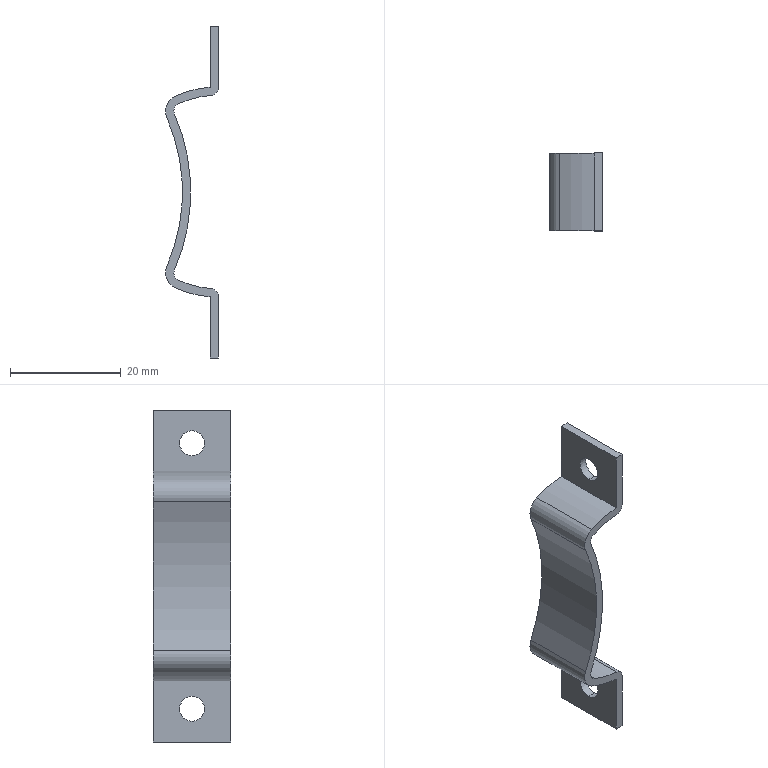Part | SolidWorks | features ExtruThin 1, ICE 1 | 1 solid | 24 faces | box 9.547 x 14 x 60 mm | volume 1466 mm3 | cylinder 16 | plane 8 | commonest cylinder face diameters 3 x4 4.5 x4 6 x2 35 x2 38 x2 67 x1
STEP:
#1=CARTESIAN_POINT('',(-1.5,7.,-26.25));
#2=VERTEX_POINT('',#1);
#3=CARTESIAN_POINT('',(-1.5,7.,-21.75));
#4=VERTEX_POINT('',#3);
#5=CARTESIAN_POINT('',(-1.5,7.,-24.));
#6=DIRECTION('',(-1.,0.,0.));
#7=DIRECTION('',(0.,0.,-1.));
#8=AXIS2_PLACEMENT_3D('',#5,#6,#7);
#9=CIRCLE('',#8,2.25);
#10=EDGE_CURVE('',#2,#4,#9,.T.);
#11=ORIENTED_EDGE('',*,*,#10,.T.);
#12=CARTESIAN_POINT('',(0.,7.,-21.75));
#13=VERTEX_POINT('',#12);
#14=CARTESIAN_POINT('',(-9.548,7.,-21.75));
#15=DIRECTION('',(1.,0.,0.));
#16=VECTOR('',#15,1000.);
#17=LINE('',#14,#16);
#18=EDGE_CURVE('',#4,#13,#17,.T.);
#19=ORIENTED_EDGE('',*,*,#18,.T.);
#20=CARTESIAN_POINT('',(0.,7.,-26.25));
#21=VERTEX_POINT('',#20);
#22=CARTESIAN_POINT('',(0.,7.,-24.));
#23=DIRECTION('',(1.,0.,0.));
#24=DIRECTION('',(0.,0.,-1.));
#25=AXIS2_PLACEMENT_3D('',#22,#23,#24);
#26=CIRCLE('',#25,2.25);
#27=EDGE_CURVE('',#13,#21,#26,.T.);
#28=ORIENTED_EDGE('',*,*,#27,.T.);
#29=CARTESIAN_POINT('',(-9.548,7.,-26.25));
#30=DIRECTION('',(1.,0.,0.));
#31=VECTOR('',#30,1000.);
#32=LINE('',#29,#31);
#33=EDGE_CURVE('',#2,#21,#32,.T.);
#34=ORIENTED_EDGE('',*,*,#33,.F.);
#35=EDGE_LOOP('',(#11,#19,#28,#34));
#36=FACE_OUTER_BOUND('',#35,.T.);
#37=CARTESIAN_POINT('',(-9.548,7.,-24.));
#38=DIRECTION('',(1.,0.,0.));
#39=DIRECTION('',(0.,0.,-1.));
#40=AXIS2_PLACEMENT_3D('',#37,#38,#39);
#41=CYLINDRICAL_SURFACE('',#40,2.25);
#42=ADVANCED_FACE('',(#36),#41,.F.);
#43=CARTESIAN_POINT('',(-1.5,7.,21.75));
#44=VERTEX_POINT('',#43);
#45=CARTESIAN_POINT('',(-1.5,7.,26.25));
#46=VERTEX_POINT('',#45);
#47=CARTESIAN_POINT('',(-1.5,7.,24.));
#48=DIRECTION('',(-1.,0.,0.));
#49=DIRECTION('',(0.,0.,-1.));
#50=AXIS2_PLACEMENT_3D('',#47,#48,#49);
#51=CIRCLE('',#50,2.25);
#52=EDGE_CURVE('',#44,#46,#51,.T.);
#53=ORIENTED_EDGE('',*,*,#52,.T.);
#54=CARTESIAN_POINT('',(0.,7.,26.25));
#55=VERTEX_POINT('',#54);
#56=CARTESIAN_POINT('',(-9.548,7.,26.25));
#57=DIRECTION('',(1.,0.,0.));
#58=VECTOR('',#57,1000.);
#59=LINE('',#56,#58);
#60=EDGE_CURVE('',#46,#55,#59,.T.);
#61=ORIENTED_EDGE('',*,*,#60,.T.);
#62=CARTESIAN_POINT('',(0.,7.,21.75));
#63=VERTEX_POINT('',#62);
#64=CARTESIAN_POINT('',(0.,7.,24.));
#65=DIRECTION('',(1.,0.,0.));
#66=DIRECTION('',(0.,0.,-1.));
#67=AXIS2_PLACEMENT_3D('',#64,#65,#66);
#68=CIRCLE('',#67,2.25);
#69=EDGE_CURVE('',#55,#63,#68,.T.);
#70=ORIENTED_EDGE('',*,*,#69,.T.);
#71=CARTESIAN_POINT('',(-9.548,7.,21.75));
#72=DIRECTION('',(1.,0.,0.));
#73=VECTOR('',#72,1000.);
#74=LINE('',#71,#73);
#75=EDGE_CURVE('',#44,#63,#74,.T.);
#76=ORIENTED_EDGE('',*,*,#75,.F.);
#77=EDGE_LOOP('',(#53,#61,#70,#76));
#78=FACE_OUTER_BOUND('',#77,.T.);
#79=CARTESIAN_POINT('',(-9.548,7.,24.));
#80=DIRECTION('',(1.,0.,0.));
#81=DIRECTION('',(0.,0.,-1.));
#82=AXIS2_PLACEMENT_3D('',#79,#80,#81);
#83=CYLINDRICAL_SURFACE('',#82,2.25);
#84=ADVANCED_FACE('',(#78),#83,.F.);
#85=ORIENTED_EDGE('',*,*,#52,.F.);
#86=CARTESIAN_POINT('',(-1.5,7.,24.));
#87=DIRECTION('',(-1.,0.,0.));
#88=DIRECTION('',(0.,0.,-1.));
#89=AXIS2_PLACEMENT_3D('',#86,#87,#88);
#90=CIRCLE('',#89,2.25);
#91=EDGE_CURVE('',#46,#44,#90,.T.);
#92=ORIENTED_EDGE('',*,*,#91,.F.);
#93=EDGE_LOOP('',(#85,#92));
#94=FACE_BOUND('',#93,.T.);
#95=CARTESIAN_POINT('',(-1.5,0.,18.941));
#96=VERTEX_POINT('',#95);
#97=CARTESIAN_POINT('',(-1.5,0.,30.));
#98=VERTEX_POINT('',#97);
#99=CARTESIAN_POINT('',(-1.5,0.,18.941));
#100=DIRECTION('',(0.,0.,1.));
#101=VECTOR('',#100,1000.);
#102=LINE('',#99,#101);
#103=EDGE_CURVE('',#96,#98,#102,.T.);
#104=ORIENTED_EDGE('',*,*,#103,.T.);
#105=CARTESIAN_POINT('',(-1.5,14.,30.));
#106=VERTEX_POINT('',#105);
#107=CARTESIAN_POINT('',(-1.5,14.,30.));
#108=DIRECTION('',(0.,-1.,0.));
#109=VECTOR('',#108,1000.);
#110=LINE('',#107,#109);
#111=EDGE_CURVE('',#106,#98,#110,.T.);
#112=ORIENTED_EDGE('',*,*,#111,.F.);
#113=CARTESIAN_POINT('',(-1.5,14.,18.941));
#114=VERTEX_POINT('',#113);
#115=CARTESIAN_POINT('',(-1.5,14.,18.941));
#116=DIRECTION('',(0.,0.,1.));
#117=VECTOR('',#116,1000.);
#118=LINE('',#115,#117);
#119=EDGE_CURVE('',#114,#106,#118,.T.);
#120=ORIENTED_EDGE('',*,*,#119,.F.);
#121=CARTESIAN_POINT('',(-1.5,14.,18.941));
#122=DIRECTION('',(0.,-1.,0.));
#123=VECTOR('',#122,1000.);
#124=LINE('',#121,#123);
#125=EDGE_CURVE('',#114,#96,#124,.T.);
#126=ORIENTED_EDGE('',*,*,#125,.T.);
#127=EDGE_LOOP('',(#104,#112,#120,#126));
#128=FACE_OUTER_BOUND('',#127,.T.);
#129=CARTESIAN_POINT('',(-1.5,14.,18.941));
#130=DIRECTION('',(1.,0.,0.));
#131=DIRECTION('',(0.,0.,-1.));
#132=AXIS2_PLACEMENT_3D('',#129,#130,#131);
#133=PLANE('',#132);
#134=ADVANCED_FACE('',(#94,#128),#133,.F.);
#135=CARTESIAN_POINT('',(0.,0.,30.));
#136=VERTEX_POINT('',#135);
#137=CARTESIAN_POINT('',(0.,0.,30.));
#138=DIRECTION('',(-1.,0.,0.));
#139=VECTOR('',#138,1000.);
#140=LINE('',#137,#139);
#141=EDGE_CURVE('',#136,#98,#140,.T.);
#142=ORIENTED_EDGE('',*,*,#141,.F.);
#143=CARTESIAN_POINT('',(0.,14.,30.));
#144=VERTEX_POINT('',#143);
#145=CARTESIAN_POINT('',(0.,14.,30.));
#146=DIRECTION('',(0.,-1.,0.));
#147=VECTOR('',#146,1000.);
#148=LINE('',#145,#147);
#149=EDGE_CURVE('',#144,#136,#148,.T.);
#150=ORIENTED_EDGE('',*,*,#149,.F.);
#151=CARTESIAN_POINT('',(0.,14.,30.));
#152=DIRECTION('',(-1.,0.,0.));
#153=VECTOR('',#152,1000.);
#154=LINE('',#151,#153);
#155=EDGE_CURVE('',#144,#106,#154,.T.);
#156=ORIENTED_EDGE('',*,*,#155,.T.);
#157=ORIENTED_EDGE('',*,*,#111,.T.);
#158=EDGE_LOOP('',(#142,#150,#156,#157));
#159=FACE_OUTER_BOUND('',#158,.T.);
#160=CARTESIAN_POINT('',(0.,14.,30.));
#161=DIRECTION('',(0.,0.,1.));
#162=DIRECTION('',(1.,0.,0.));
#163=AXIS2_PLACEMENT_3D('',#160,#161,#162);
#164=PLANE('',#163);
#165=ADVANCED_FACE('',(#159),#164,.T.);
#166=CARTESIAN_POINT('',(0.,7.,24.));
#167=DIRECTION('',(1.,0.,0.));
#168=DIRECTION('',(0.,0.,-1.));
#169=AXIS2_PLACEMENT_3D('',#166,#167,#168);
#170=CIRCLE('',#169,2.25);
#171=EDGE_CURVE('',#63,#55,#170,.T.);
#172=ORIENTED_EDGE('',*,*,#171,.F.);
#173=ORIENTED_EDGE('',*,*,#69,.F.);
#174=EDGE_LOOP('',(#172,#173));
#175=FACE_BOUND('',#174,.T.);
#176=CARTESIAN_POINT('',(0.,0.,18.941));
#177=VERTEX_POINT('',#176);
#178=CARTESIAN_POINT('',(0.,0.,18.941));
#179=DIRECTION('',(0.,0.,1.));
#180=VECTOR('',#179,1000.);
#181=LINE('',#178,#180);
#182=EDGE_CURVE('',#177,#136,#181,.T.);
#183=ORIENTED_EDGE('',*,*,#182,.F.);
#184=CARTESIAN_POINT('',(0.,14.,18.941));
#185=VERTEX_POINT('',#184);
#186=CARTESIAN_POINT('',(0.,14.,18.941));
#187=DIRECTION('',(0.,-1.,0.));
#188=VECTOR('',#187,1000.);
#189=LINE('',#186,#188);
#190=EDGE_CURVE('',#185,#177,#189,.T.);
#191=ORIENTED_EDGE('',*,*,#190,.F.);
#192=CARTESIAN_POINT('',(0.,14.,18.941));
#193=DIRECTION('',(0.,0.,1.));
#194=VECTOR('',#193,1000.);
#195=LINE('',#192,#194);
#196=EDGE_CURVE('',#185,#144,#195,.T.);
#197=ORIENTED_EDGE('',*,*,#196,.T.);
#198=ORIENTED_EDGE('',*,*,#149,.T.);
#199=EDGE_LOOP('',(#183,#191,#197,#198));
#200=FACE_OUTER_BOUND('',#199,.T.);
#201=CARTESIAN_POINT('',(0.,14.,18.941));
#202=DIRECTION('',(1.,0.,0.));
#203=DIRECTION('',(0.,0.,-1.));
#204=AXIS2_PLACEMENT_3D('',#201,#202,#203);
#205=PLANE('',#204);
#206=ADVANCED_FACE('',(#175,#200),#205,.T.);
#207=CARTESIAN_POINT('',(-1.382,0.,17.445));
#208=VERTEX_POINT('',#207);
#209=CARTESIAN_POINT('',(-1.5,0.,18.941));
#210=DIRECTION('',(0.,-1.,0.));
#211=DIRECTION('',(0.,0.,1.));
#212=AXIS2_PLACEMENT_3D('',#209,#210,#211);
#213=CIRCLE('',#212,1.5);
#214=EDGE_CURVE('',#208,#177,#213,.T.);
#215=ORIENTED_EDGE('',*,*,#214,.F.);
#216=CARTESIAN_POINT('',(-1.382,14.,17.445));
#217=VERTEX_POINT('',#216);
#218=CARTESIAN_POINT('',(-1.382,14.,17.445));
#219=DIRECTION('',(0.,-1.,0.));
#220=VECTOR('',#219,1000.);
#221=LINE('',#218,#220);
#222=EDGE_CURVE('',#217,#208,#221,.T.);
#223=ORIENTED_EDGE('',*,*,#222,.F.);
#224=CARTESIAN_POINT('',(-1.5,14.,18.941));
#225=DIRECTION('',(0.,-1.,0.));
#226=DIRECTION('',(0.,0.,1.));
#227=AXIS2_PLACEMENT_3D('',#224,#225,#226);
#228=CIRCLE('',#227,1.5);
#229=EDGE_CURVE('',#217,#185,#228,.T.);
#230=ORIENTED_EDGE('',*,*,#229,.T.);
#231=ORIENTED_EDGE('',*,*,#190,.T.);
#232=EDGE_LOOP('',(#215,#223,#230,#231));
#233=FACE_OUTER_BOUND('',#232,.T.);
#234=CARTESIAN_POINT('',(-1.5,14.,18.941));
#235=DIRECTION('',(0.,-1.,0.));
#236=DIRECTION('',(0.,0.,-1.));
#237=AXIS2_PLACEMENT_3D('',#234,#235,#236);
#238=CYLINDRICAL_SURFACE('',#237,1.5);
#239=ADVANCED_FACE('',(#233),#238,.T.);
#240=CARTESIAN_POINT('',(-7.161,0.,15.968));
#241=VERTEX_POINT('',#240);
#242=CARTESIAN_POINT('',(0.,0.,0.));
#243=DIRECTION('',(0.,1.,0.));
#244=DIRECTION('',(0.,0.,1.));
#245=AXIS2_PLACEMENT_3D('',#242,#243,#244);
#246=CIRCLE('',#245,17.5);
#247=EDGE_CURVE('',#241,#208,#246,.T.);
#248=ORIENTED_EDGE('',*,*,#247,.F.);
#249=CARTESIAN_POINT('',(-7.161,14.,15.968));
#250=VERTEX_POINT('',#249);
#251=CARTESIAN_POINT('',(-7.161,14.,15.968));
#252=DIRECTION('',(0.,-1.,0.));
#253=VECTOR('',#252,1000.);
#254=LINE('',#251,#253);
#255=EDGE_CURVE('',#250,#241,#254,.T.);
#256=ORIENTED_EDGE('',*,*,#255,.F.);
#257=CARTESIAN_POINT('',(0.,14.,0.));
#258=DIRECTION('',(0.,1.,0.));
#259=DIRECTION('',(0.,0.,1.));
#260=AXIS2_PLACEMENT_3D('',#257,#258,#259);
#261=CIRCLE('',#260,17.5);
#262=EDGE_CURVE('',#250,#217,#261,.T.);
#263=ORIENTED_EDGE('',*,*,#262,.T.);
#264=ORIENTED_EDGE('',*,*,#222,.T.);
#265=EDGE_LOOP('',(#248,#256,#263,#264));
#266=FACE_OUTER_BOUND('',#265,.T.);
#267=CARTESIAN_POINT('',(0.,14.,0.));
#268=DIRECTION('',(0.,-1.,0.));
#269=DIRECTION('',(0.,0.,-1.));
#270=AXIS2_PLACEMENT_3D('',#267,#268,#269);
#271=CYLINDRICAL_SURFACE('',#270,17.5);
#272=ADVANCED_FACE('',(#266),#271,.F.);
#273=CARTESIAN_POINT('',(-7.922,0.,13.999));
#274=VERTEX_POINT('',#273);
#275=CARTESIAN_POINT('',(-6.547,0.,14.599));
#276=DIRECTION('',(0.,1.,0.));
#277=DIRECTION('',(0.,0.,-1.));
#278=AXIS2_PLACEMENT_3D('',#275,#276,#277);
#279=CIRCLE('',#278,1.5);
#280=EDGE_CURVE('',#274,#241,#279,.T.);
#281=ORIENTED_EDGE('',*,*,#280,.F.);
#282=CARTESIAN_POINT('',(-7.922,14.,13.999));
#283=VERTEX_POINT('',#282);
#284=CARTESIAN_POINT('',(-7.922,14.,13.999));
#285=DIRECTION('',(0.,-1.,0.));
#286=VECTOR('',#285,1000.);
#287=LINE('',#284,#286);
#288=EDGE_CURVE('',#283,#274,#287,.T.);
#289=ORIENTED_EDGE('',*,*,#288,.F.);
#290=CARTESIAN_POINT('',(-6.547,14.,14.599));
#291=DIRECTION('',(0.,1.,0.));
#292=DIRECTION('',(0.,0.,-1.));
#293=AXIS2_PLACEMENT_3D('',#290,#291,#292);
#294=CIRCLE('',#293,1.5);
#295=EDGE_CURVE('',#283,#250,#294,.T.);
#296=ORIENTED_EDGE('',*,*,#295,.T.);
#297=ORIENTED_EDGE('',*,*,#255,.T.);
#298=EDGE_LOOP('',(#281,#289,#296,#297));
#299=FACE_OUTER_BOUND('',#298,.T.);
#300=CARTESIAN_POINT('',(-6.547,14.,14.599));
#301=DIRECTION('',(0.,-1.,0.));
#302=DIRECTION('',(0.,0.,-1.));
#303=AXIS2_PLACEMENT_3D('',#300,#301,#302);
#304=CYLINDRICAL_SURFACE('',#303,1.5);
#305=ADVANCED_FACE('',(#299),#304,.F.);
#306=CARTESIAN_POINT('',(-7.922,0.,-13.999));
#307=VERTEX_POINT('',#306);
#308=CARTESIAN_POINT('',(-40.,0.,0.));
#309=DIRECTION('',(0.,-1.,0.));
#310=DIRECTION('',(0.,0.,1.));
#311=AXIS2_PLACEMENT_3D('',#308,#309,#310);
#312=CIRCLE('',#311,35.);
#313=EDGE_CURVE('',#307,#274,#312,.T.);
#314=ORIENTED_EDGE('',*,*,#313,.F.);
#315=CARTESIAN_POINT('',(-7.922,14.,-13.999));
#316=VERTEX_POINT('',#315);
#317=CARTESIAN_POINT('',(-7.922,14.,-13.999));
#318=DIRECTION('',(0.,-1.,0.));
#319=VECTOR('',#318,1000.);
#320=LINE('',#317,#319);
#321=EDGE_CURVE('',#316,#307,#320,.T.);
#322=ORIENTED_EDGE('',*,*,#321,.F.);
#323=CARTESIAN_POINT('',(-40.,14.,0.));
#324=DIRECTION('',(0.,-1.,0.));
#325=DIRECTION('',(0.,0.,1.));
#326=AXIS2_PLACEMENT_3D('',#323,#324,#325);
#327=CIRCLE('',#326,35.);
#328=EDGE_CURVE('',#316,#283,#327,.T.);
#329=ORIENTED_EDGE('',*,*,#328,.T.);
#330=ORIENTED_EDGE('',*,*,#288,.T.);
#331=EDGE_LOOP('',(#314,#322,#329,#330));
#332=FACE_OUTER_BOUND('',#331,.T.);
#333=CARTESIAN_POINT('',(-40.,14.,0.));
#334=DIRECTION('',(0.,-1.,0.));
#335=DIRECTION('',(0.,0.,-1.));
#336=AXIS2_PLACEMENT_3D('',#333,#334,#335);
#337=CYLINDRICAL_SURFACE('',#336,35.);
#338=ADVANCED_FACE('',(#332),#337,.T.);
#339=CARTESIAN_POINT('',(-7.161,0.,-15.968));
#340=VERTEX_POINT('',#339);
#341=CARTESIAN_POINT('',(-6.547,0.,-14.599));
#342=DIRECTION('',(0.,1.,0.));
#343=DIRECTION('',(0.,0.,-1.));
#344=AXIS2_PLACEMENT_3D('',#341,#342,#343);
#345=CIRCLE('',#344,1.5);
#346=EDGE_CURVE('',#340,#307,#345,.T.);
#347=ORIENTED_EDGE('',*,*,#346,.F.);
#348=CARTESIAN_POINT('',(-7.161,14.,-15.968));
#349=VERTEX_POINT('',#348);
#350=CARTESIAN_POINT('',(-7.161,14.,-15.968));
#351=DIRECTION('',(0.,-1.,0.));
#352=VECTOR('',#351,1000.);
#353=LINE('',#350,#352);
#354=EDGE_CURVE('',#349,#340,#353,.T.);
#355=ORIENTED_EDGE('',*,*,#354,.F.);
#356=CARTESIAN_POINT('',(-6.547,14.,-14.599));
#357=DIRECTION('',(0.,1.,0.));
#358=DIRECTION('',(0.,0.,-1.));
#359=AXIS2_PLACEMENT_3D('',#356,#357,#358);
#360=CIRCLE('',#359,1.5);
#361=EDGE_CURVE('',#349,#316,#360,.T.);
#362=ORIENTED_EDGE('',*,*,#361,.T.);
#363=ORIENTED_EDGE('',*,*,#321,.T.);
#364=EDGE_LOOP('',(#347,#355,#362,#363));
#365=FACE_OUTER_BOUND('',#364,.T.);
#366=CARTESIAN_POINT('',(-6.547,14.,-14.599));
#367=DIRECTION('',(0.,-1.,0.));
#368=DIRECTION('',(0.,0.,-1.));
#369=AXIS2_PLACEMENT_3D('',#366,#367,#368);
#370=CYLINDRICAL_SURFACE('',#369,1.5);
#371=ADVANCED_FACE('',(#365),#370,.F.);
#372=CARTESIAN_POINT('',(-1.382,0.,-17.445));
#373=VERTEX_POINT('',#372);
#374=CARTESIAN_POINT('',(0.,0.,0.));
#375=DIRECTION('',(0.,1.,0.));
#376=DIRECTION('',(0.,0.,1.));
#377=AXIS2_PLACEMENT_3D('',#374,#375,#376);
#378=CIRCLE('',#377,17.5);
#379=EDGE_CURVE('',#373,#340,#378,.T.);
#380=ORIENTED_EDGE('',*,*,#379,.F.);
#381=CARTESIAN_POINT('',(-1.382,14.,-17.445));
#382=VERTEX_POINT('',#381);
#383=CARTESIAN_POINT('',(-1.382,14.,-17.445));
#384=DIRECTION('',(0.,-1.,0.));
#385=VECTOR('',#384,1000.);
#386=LINE('',#383,#385);
#387=EDGE_CURVE('',#382,#373,#386,.T.);
#388=ORIENTED_EDGE('',*,*,#387,.F.);
#389=CARTESIAN_POINT('',(0.,14.,0.));
#390=DIRECTION('',(0.,1.,0.));
#391=DIRECTION('',(0.,0.,1.));
#392=AXIS2_PLACEMENT_3D('',#389,#390,#391);
#393=CIRCLE('',#392,17.5);
#394=EDGE_CURVE('',#382,#349,#393,.T.);
#395=ORIENTED_EDGE('',*,*,#394,.T.);
#396=ORIENTED_EDGE('',*,*,#354,.T.);
#397=EDGE_LOOP('',(#380,#388,#395,#396));
#398=FACE_OUTER_BOUND('',#397,.T.);
#399=CARTESIAN_POINT('',(0.,14.,0.));
#400=DIRECTION('',(0.,-1.,0.));
#401=DIRECTION('',(0.,0.,-1.));
#402=AXIS2_PLACEMENT_3D('',#399,#400,#401);
#403=CYLINDRICAL_SURFACE('',#402,17.5);
#404=ADVANCED_FACE('',(#398),#403,.F.);
#405=CARTESIAN_POINT('',(0.,0.,-18.941));
#406=VERTEX_POINT('',#405);
#407=CARTESIAN_POINT('',(-1.5,0.,-18.941));
#408=DIRECTION('',(0.,-1.,0.));
#409=DIRECTION('',(0.,0.,-1.));
#410=AXIS2_PLACEMENT_3D('',#407,#408,#409);
#411=CIRCLE('',#410,1.5);
#412=EDGE_CURVE('',#406,#373,#411,.T.);
#413=ORIENTED_EDGE('',*,*,#412,.F.);
#414=CARTESIAN_POINT('',(0.,14.,-18.941));
#415=VERTEX_POINT('',#414);
#416=CARTESIAN_POINT('',(0.,14.,-18.941));
#417=DIRECTION('',(0.,-1.,0.));
#418=VECTOR('',#417,1000.);
#419=LINE('',#416,#418);
#420=EDGE_CURVE('',#415,#406,#419,.T.);
#421=ORIENTED_EDGE('',*,*,#420,.F.);
#422=CARTESIAN_POINT('',(-1.5,14.,-18.941));
#423=DIRECTION('',(0.,-1.,0.));
#424=DIRECTION('',(0.,0.,-1.));
#425=AXIS2_PLACEMENT_3D('',#422,#423,#424);
#426=CIRCLE('',#425,1.5);
#427=EDGE_CURVE('',#415,#382,#426,.T.);
#428=ORIENTED_EDGE('',*,*,#427,.T.);
#429=ORIENTED_EDGE('',*,*,#387,.T.);
#430=EDGE_LOOP('',(#413,#421,#428,#429));
#431=FACE_OUTER_BOUND('',#430,.T.);
#432=CARTESIAN_POINT('',(-1.5,14.,-18.941));
#433=DIRECTION('',(0.,-1.,0.));
#434=DIRECTION('',(0.,0.,-1.));
#435=AXIS2_PLACEMENT_3D('',#432,#433,#434);
#436=CYLINDRICAL_SURFACE('',#435,1.5);
#437=ADVANCED_FACE('',(#431),#436,.T.);
#438=CARTESIAN_POINT('',(0.,7.,-24.));
#439=DIRECTION('',(1.,0.,0.));
#440=DIRECTION('',(0.,0.,-1.));
#441=AXIS2_PLACEMENT_3D('',#438,#439,#440);
#442=CIRCLE('',#441,2.25);
#443=EDGE_CURVE('',#21,#13,#442,.T.);
#444=ORIENTED_EDGE('',*,*,#443,.F.);
#445=ORIENTED_EDGE('',*,*,#27,.F.);
#446=EDGE_LOOP('',(#444,#445));
#447=FACE_BOUND('',#446,.T.);
#448=CARTESIAN_POINT('',(0.,0.,-30.));
#449=VERTEX_POINT('',#448);
#450=CARTESIAN_POINT('',(0.,0.,-18.941));
#451=DIRECTION('',(0.,0.,1.));
#452=VECTOR('',#451,1000.);
#453=LINE('',#450,#452);
#454=EDGE_CURVE('',#449,#406,#453,.T.);
#455=ORIENTED_EDGE('',*,*,#454,.F.);
#456=CARTESIAN_POINT('',(0.,14.,-30.));
#457=VERTEX_POINT('',#456);
#458=CARTESIAN_POINT('',(0.,14.,-30.));
#459=DIRECTION('',(0.,-1.,0.));
#460=VECTOR('',#459,1000.);
#461=LINE('',#458,#460);
#462=EDGE_CURVE('',#457,#449,#461,.T.);
#463=ORIENTED_EDGE('',*,*,#462,.F.);
#464=CARTESIAN_POINT('',(0.,14.,-18.941));
#465=DIRECTION('',(0.,0.,1.));
#466=VECTOR('',#465,1000.);
#467=LINE('',#464,#466);
#468=EDGE_CURVE('',#457,#415,#467,.T.);
#469=ORIENTED_EDGE('',*,*,#468,.T.);
#470=ORIENTED_EDGE('',*,*,#420,.T.);
#471=EDGE_LOOP('',(#455,#463,#469,#470));
#472=FACE_OUTER_BOUND('',#471,.T.);
#473=CARTESIAN_POINT('',(0.,14.,-18.941));
#474=DIRECTION('',(1.,0.,0.));
#475=DIRECTION('',(0.,0.,-1.));
#476=AXIS2_PLACEMENT_3D('',#473,#474,#475);
#477=PLANE('',#476);
#478=ADVANCED_FACE('',(#447,#472),#477,.T.);
#479=CARTESIAN_POINT('',(-1.5,0.,-30.));
#480=VERTEX_POINT('',#479);
#481=CARTESIAN_POINT('',(-1.5,0.,-30.));
#482=DIRECTION('',(1.,0.,0.));
#483=VECTOR('',#482,1000.);
#484=LINE('',#481,#483);
#485=EDGE_CURVE('',#480,#449,#484,.T.);
#486=ORIENTED_EDGE('',*,*,#485,.F.);
#487=CARTESIAN_POINT('',(-1.5,14.,-30.));
#488=VERTEX_POINT('',#487);
#489=CARTESIAN_POINT('',(-1.5,14.,-30.));
#490=DIRECTION('',(0.,-1.,0.));
#491=VECTOR('',#490,1000.);
#492=LINE('',#489,#491);
#493=EDGE_CURVE('',#488,#480,#492,.T.);
#494=ORIENTED_EDGE('',*,*,#493,.F.);
#495=CARTESIAN_POINT('',(-1.5,14.,-30.));
#496=DIRECTION('',(1.,0.,0.));
#497=VECTOR('',#496,1000.);
#498=LINE('',#495,#497);
#499=EDGE_CURVE('',#488,#457,#498,.T.);
#500=ORIENTED_EDGE('',*,*,#499,.T.);
#501=ORIENTED_EDGE('',*,*,#462,.T.);
#502=EDGE_LOOP('',(#486,#494,#500,#501));
#503=FACE_OUTER_BOUND('',#502,.T.);
#504=CARTESIAN_POINT('',(-1.5,14.,-30.));
#505=DIRECTION('',(0.,0.,-1.));
#506=DIRECTION('',(-1.,0.,0.));
#507=AXIS2_PLACEMENT_3D('',#504,#505,#506);
#508=PLANE('',#507);
#509=ADVANCED_FACE('',(#503),#508,.T.);
#510=ORIENTED_EDGE('',*,*,#10,.F.);
#511=CARTESIAN_POINT('',(-1.5,7.,-24.));
#512=DIRECTION('',(-1.,0.,0.));
#513=DIRECTION('',(0.,0.,-1.));
#514=AXIS2_PLACEMENT_3D('',#511,#512,#513);
#515=CIRCLE('',#514,2.25);
#516=EDGE_CURVE('',#4,#2,#515,.T.);
#517=ORIENTED_EDGE('',*,*,#516,.F.);
#518=EDGE_LOOP('',(#510,#517));
#519=FACE_BOUND('',#518,.T.);
#520=CARTESIAN_POINT('',(-1.5,0.,-18.941));
#521=VERTEX_POINT('',#520);
#522=CARTESIAN_POINT('',(-1.5,0.,-18.941));
#523=DIRECTION('',(0.,0.,1.));
#524=VECTOR('',#523,1000.);
#525=LINE('',#522,#524);
#526=EDGE_CURVE('',#480,#521,#525,.T.);
#527=ORIENTED_EDGE('',*,*,#526,.T.);
#528=CARTESIAN_POINT('',(-1.5,14.,-18.941));
#529=VERTEX_POINT('',#528);
#530=CARTESIAN_POINT('',(-1.5,14.,-18.941));
#531=DIRECTION('',(0.,-1.,0.));
#532=VECTOR('',#531,1000.);
#533=LINE('',#530,#532);
#534=EDGE_CURVE('',#529,#521,#533,.T.);
#535=ORIENTED_EDGE('',*,*,#534,.F.);
#536=CARTESIAN_POINT('',(-1.5,14.,-18.941));
#537=DIRECTION('',(0.,0.,1.));
#538=VECTOR('',#537,1000.);
#539=LINE('',#536,#538);
#540=EDGE_CURVE('',#488,#529,#539,.T.);
#541=ORIENTED_EDGE('',*,*,#540,.F.);
#542=ORIENTED_EDGE('',*,*,#493,.T.);
#543=EDGE_LOOP('',(#527,#535,#541,#542));
#544=FACE_OUTER_BOUND('',#543,.T.);
#545=CARTESIAN_POINT('',(-1.5,14.,-18.941));
#546=DIRECTION('',(1.,0.,0.));
#547=DIRECTION('',(0.,0.,-1.));
#548=AXIS2_PLACEMENT_3D('',#545,#546,#547);
#549=PLANE('',#548);
#550=ADVANCED_FACE('',(#519,#544),#549,.F.);
#551=CARTESIAN_POINT('',(-7.774,0.,-17.337));
#552=VERTEX_POINT('',#551);
#553=CARTESIAN_POINT('',(0.,0.,0.));
#554=DIRECTION('',(0.,1.,0.));
#555=DIRECTION('',(1.,0.,0.));
#556=AXIS2_PLACEMENT_3D('',#553,#554,#555);
#557=CIRCLE('',#556,19.);
#558=EDGE_CURVE('',#521,#552,#557,.T.);
#559=ORIENTED_EDGE('',*,*,#558,.T.);
#560=CARTESIAN_POINT('',(-7.774,14.,-17.337));
#561=VERTEX_POINT('',#560);
#562=CARTESIAN_POINT('',(-7.774,14.,-17.337));
#563=DIRECTION('',(0.,-1.,0.));
#564=VECTOR('',#563,1000.);
#565=LINE('',#562,#564);
#566=EDGE_CURVE('',#561,#552,#565,.T.);
#567=ORIENTED_EDGE('',*,*,#566,.F.);
#568=CARTESIAN_POINT('',(0.,14.,0.));
#569=DIRECTION('',(0.,1.,0.));
#570=DIRECTION('',(1.,0.,0.));
#571=AXIS2_PLACEMENT_3D('',#568,#569,#570);
#572=CIRCLE('',#571,19.);
#573=EDGE_CURVE('',#529,#561,#572,.T.);
#574=ORIENTED_EDGE('',*,*,#573,.F.);
#575=ORIENTED_EDGE('',*,*,#534,.T.);
#576=EDGE_LOOP('',(#559,#567,#574,#575));
#577=FACE_OUTER_BOUND('',#576,.T.);
#578=CARTESIAN_POINT('',(0.,14.,0.));
#579=DIRECTION('',(0.,-1.,0.));
#580=DIRECTION('',(0.,0.,-1.));
#581=AXIS2_PLACEMENT_3D('',#578,#579,#580);
#582=CYLINDRICAL_SURFACE('',#581,19.);
#583=ADVANCED_FACE('',(#577),#582,.T.);
#584=CARTESIAN_POINT('',(-9.296,0.,-13.399));
#585=VERTEX_POINT('',#584);
#586=CARTESIAN_POINT('',(-6.547,0.,-14.599));
#587=DIRECTION('',(0.,1.,0.));
#588=DIRECTION('',(1.,0.,0.));
#589=AXIS2_PLACEMENT_3D('',#586,#587,#588);
#590=CIRCLE('',#589,3.);
#591=EDGE_CURVE('',#552,#585,#590,.T.);
#592=ORIENTED_EDGE('',*,*,#591,.T.);
#593=CARTESIAN_POINT('',(-9.296,14.,-13.399));
#594=VERTEX_POINT('',#593);
#595=CARTESIAN_POINT('',(-9.296,14.,-13.399));
#596=DIRECTION('',(0.,-1.,0.));
#597=VECTOR('',#596,1000.);
#598=LINE('',#595,#597);
#599=EDGE_CURVE('',#594,#585,#598,.T.);
#600=ORIENTED_EDGE('',*,*,#599,.F.);
#601=CARTESIAN_POINT('',(-6.547,14.,-14.599));
#602=DIRECTION('',(0.,1.,0.));
#603=DIRECTION('',(1.,0.,0.));
#604=AXIS2_PLACEMENT_3D('',#601,#602,#603);
#605=CIRCLE('',#604,3.);
#606=EDGE_CURVE('',#561,#594,#605,.T.);
#607=ORIENTED_EDGE('',*,*,#606,.F.);
#608=ORIENTED_EDGE('',*,*,#566,.T.);
#609=EDGE_LOOP('',(#592,#600,#607,#608));
#610=FACE_OUTER_BOUND('',#609,.T.);
#611=CARTESIAN_POINT('',(-6.547,14.,-14.599));
#612=DIRECTION('',(0.,-1.,0.));
#613=DIRECTION('',(0.,0.,-1.));
#614=AXIS2_PLACEMENT_3D('',#611,#612,#613);
#615=CYLINDRICAL_SURFACE('',#614,3.);
#616=ADVANCED_FACE('',(#610),#615,.T.);
#617=CARTESIAN_POINT('',(-9.296,0.,13.399));
#618=VERTEX_POINT('',#617);
#619=CARTESIAN_POINT('',(-40.,0.,0.));
#620=DIRECTION('',(0.,-1.,0.));
#621=DIRECTION('',(1.,0.,0.));
#622=AXIS2_PLACEMENT_3D('',#619,#620,#621);
#623=CIRCLE('',#622,33.5);
#624=EDGE_CURVE('',#585,#618,#623,.T.);
#625=ORIENTED_EDGE('',*,*,#624,.T.);
#626=CARTESIAN_POINT('',(-9.296,14.,13.399));
#627=VERTEX_POINT('',#626);
#628=CARTESIAN_POINT('',(-9.296,14.,13.399));
#629=DIRECTION('',(0.,-1.,0.));
#630=VECTOR('',#629,1000.);
#631=LINE('',#628,#630);
#632=EDGE_CURVE('',#627,#618,#631,.T.);
#633=ORIENTED_EDGE('',*,*,#632,.F.);
#634=CARTESIAN_POINT('',(-40.,14.,0.));
#635=DIRECTION('',(0.,-1.,0.));
#636=DIRECTION('',(1.,0.,0.));
#637=AXIS2_PLACEMENT_3D('',#634,#635,#636);
#638=CIRCLE('',#637,33.5);
#639=EDGE_CURVE('',#594,#627,#638,.T.);
#640=ORIENTED_EDGE('',*,*,#639,.F.);
#641=ORIENTED_EDGE('',*,*,#599,.T.);
#642=EDGE_LOOP('',(#625,#633,#640,#641));
#643=FACE_OUTER_BOUND('',#642,.T.);
#644=CARTESIAN_POINT('',(-40.,14.,0.));
#645=DIRECTION('',(0.,-1.,0.));
#646=DIRECTION('',(0.,0.,-1.));
#647=AXIS2_PLACEMENT_3D('',#644,#645,#646);
#648=CYLINDRICAL_SURFACE('',#647,33.5);
#649=ADVANCED_FACE('',(#643),#648,.F.);
#650=CARTESIAN_POINT('',(-7.774,0.,17.337));
#651=VERTEX_POINT('',#650);
#652=CARTESIAN_POINT('',(-6.547,0.,14.599));
#653=DIRECTION('',(0.,1.,0.));
#654=DIRECTION('',(1.,0.,0.));
#655=AXIS2_PLACEMENT_3D('',#652,#653,#654);
#656=CIRCLE('',#655,3.);
#657=EDGE_CURVE('',#618,#651,#656,.T.);
#658=ORIENTED_EDGE('',*,*,#657,.T.);
#659=CARTESIAN_POINT('',(-7.774,14.,17.337));
#660=VERTEX_POINT('',#659);
#661=CARTESIAN_POINT('',(-7.774,14.,17.337));
#662=DIRECTION('',(0.,-1.,0.));
#663=VECTOR('',#662,1000.);
#664=LINE('',#661,#663);
#665=EDGE_CURVE('',#660,#651,#664,.T.);
#666=ORIENTED_EDGE('',*,*,#665,.F.);
#667=CARTESIAN_POINT('',(-6.547,14.,14.599));
#668=DIRECTION('',(0.,1.,0.));
#669=DIRECTION('',(1.,0.,0.));
#670=AXIS2_PLACEMENT_3D('',#667,#668,#669);
#671=CIRCLE('',#670,3.);
#672=EDGE_CURVE('',#627,#660,#671,.T.);
#673=ORIENTED_EDGE('',*,*,#672,.F.);
#674=ORIENTED_EDGE('',*,*,#632,.T.);
#675=EDGE_LOOP('',(#658,#666,#673,#674));
#676=FACE_OUTER_BOUND('',#675,.T.);
#677=CARTESIAN_POINT('',(-6.547,14.,14.599));
#678=DIRECTION('',(0.,-1.,0.));
#679=DIRECTION('',(0.,0.,-1.));
#680=AXIS2_PLACEMENT_3D('',#677,#678,#679);
#681=CYLINDRICAL_SURFACE('',#680,3.);
#682=ADVANCED_FACE('',(#676),#681,.T.);
#683=CARTESIAN_POINT('',(0.,0.,0.));
#684=DIRECTION('',(0.,1.,0.));
#685=DIRECTION('',(1.,0.,0.));
#686=AXIS2_PLACEMENT_3D('',#683,#684,#685);
#687=CIRCLE('',#686,19.);
#688=EDGE_CURVE('',#651,#96,#687,.T.);
#689=ORIENTED_EDGE('',*,*,#688,.T.);
#690=ORIENTED_EDGE('',*,*,#125,.F.);
#691=CARTESIAN_POINT('',(0.,14.,0.));
#692=DIRECTION('',(0.,1.,0.));
#693=DIRECTION('',(1.,0.,0.));
#694=AXIS2_PLACEMENT_3D('',#691,#692,#693);
#695=CIRCLE('',#694,19.);
#696=EDGE_CURVE('',#660,#114,#695,.T.);
#697=ORIENTED_EDGE('',*,*,#696,.F.);
#698=ORIENTED_EDGE('',*,*,#665,.T.);
#699=EDGE_LOOP('',(#689,#690,#697,#698));
#700=FACE_OUTER_BOUND('',#699,.T.);
#701=CARTESIAN_POINT('',(0.,14.,0.));
#702=DIRECTION('',(0.,-1.,0.));
#703=DIRECTION('',(0.,0.,-1.));
#704=AXIS2_PLACEMENT_3D('',#701,#702,#703);
#705=CYLINDRICAL_SURFACE('',#704,19.);
#706=ADVANCED_FACE('',(#700),#705,.T.);
#707=ORIENTED_EDGE('',*,*,#119,.T.);
#708=ORIENTED_EDGE('',*,*,#155,.F.);
#709=ORIENTED_EDGE('',*,*,#196,.F.);
#710=ORIENTED_EDGE('',*,*,#229,.F.);
#711=ORIENTED_EDGE('',*,*,#262,.F.);
#712=ORIENTED_EDGE('',*,*,#295,.F.);
#713=ORIENTED_EDGE('',*,*,#328,.F.);
#714=ORIENTED_EDGE('',*,*,#361,.F.);
#715=ORIENTED_EDGE('',*,*,#394,.F.);
#716=ORIENTED_EDGE('',*,*,#427,.F.);
#717=ORIENTED_EDGE('',*,*,#468,.F.);
#718=ORIENTED_EDGE('',*,*,#499,.F.);
#719=ORIENTED_EDGE('',*,*,#540,.T.);
#720=ORIENTED_EDGE('',*,*,#573,.T.);
#721=ORIENTED_EDGE('',*,*,#606,.T.);
#722=ORIENTED_EDGE('',*,*,#639,.T.);
#723=ORIENTED_EDGE('',*,*,#672,.T.);
#724=ORIENTED_EDGE('',*,*,#696,.T.);
#725=EDGE_LOOP('',(#707,#708,#709,#710,#711,#712,#713,#714,#715,#716,#717,#718,#719,#720,#721,#722,#723,#724));
#726=FACE_OUTER_BOUND('',#725,.T.);
#727=CARTESIAN_POINT('',(-1.5,14.,18.941));
#728=DIRECTION('',(0.,-1.,0.));
#729=DIRECTION('',(-1.,0.,0.));
#730=AXIS2_PLACEMENT_3D('',#727,#728,#729);
#731=PLANE('',#730);
#732=ADVANCED_FACE('',(#726),#731,.F.);
#733=ORIENTED_EDGE('',*,*,#103,.F.);
#734=ORIENTED_EDGE('',*,*,#688,.F.);
#735=ORIENTED_EDGE('',*,*,#657,.F.);
#736=ORIENTED_EDGE('',*,*,#624,.F.);
#737=ORIENTED_EDGE('',*,*,#591,.F.);
#738=ORIENTED_EDGE('',*,*,#558,.F.);
#739=ORIENTED_EDGE('',*,*,#526,.F.);
#740=ORIENTED_EDGE('',*,*,#485,.T.);
#741=ORIENTED_EDGE('',*,*,#454,.T.);
#742=ORIENTED_EDGE('',*,*,#412,.T.);
#743=ORIENTED_EDGE('',*,*,#379,.T.);
#744=ORIENTED_EDGE('',*,*,#346,.T.);
#745=ORIENTED_EDGE('',*,*,#313,.T.);
#746=ORIENTED_EDGE('',*,*,#280,.T.);
#747=ORIENTED_EDGE('',*,*,#247,.T.);
#748=ORIENTED_EDGE('',*,*,#214,.T.);
#749=ORIENTED_EDGE('',*,*,#182,.T.);
#750=ORIENTED_EDGE('',*,*,#141,.T.);
#751=EDGE_LOOP('',(#733,#734,#735,#736,#737,#738,#739,#740,#741,#742,#743,#744,#745,#746,#747,#748,#749,#750));
#752=FACE_OUTER_BOUND('',#751,.T.);
#753=CARTESIAN_POINT('',(-1.5,0.,18.941));
#754=DIRECTION('',(0.,-1.,0.));
#755=DIRECTION('',(-1.,0.,0.));
#756=AXIS2_PLACEMENT_3D('',#753,#754,#755);
#757=PLANE('',#756);
#758=ADVANCED_FACE('',(#752),#757,.T.);
#759=ORIENTED_EDGE('',*,*,#60,.F.);
#760=ORIENTED_EDGE('',*,*,#91,.T.);
#761=ORIENTED_EDGE('',*,*,#75,.T.);
#762=ORIENTED_EDGE('',*,*,#171,.T.);
#763=EDGE_LOOP('',(#759,#760,#761,#762));
#764=FACE_OUTER_BOUND('',#763,.T.);
#765=CARTESIAN_POINT('',(-9.548,7.,24.));
#766=DIRECTION('',(1.,0.,0.));
#767=DIRECTION('',(0.,0.,-1.));
#768=AXIS2_PLACEMENT_3D('',#765,#766,#767);
#769=CYLINDRICAL_SURFACE('',#768,2.25);
#770=ADVANCED_FACE('',(#764),#769,.F.);
#771=ORIENTED_EDGE('',*,*,#18,.F.);
#772=ORIENTED_EDGE('',*,*,#516,.T.);
#773=ORIENTED_EDGE('',*,*,#33,.T.);
#774=ORIENTED_EDGE('',*,*,#443,.T.);
#775=EDGE_LOOP('',(#771,#772,#773,#774));
#776=FACE_OUTER_BOUND('',#775,.T.);
#777=CARTESIAN_POINT('',(-9.548,7.,-24.));
#778=DIRECTION('',(1.,0.,0.));
#779=DIRECTION('',(0.,0.,-1.));
#780=AXIS2_PLACEMENT_3D('',#777,#778,#779);
#781=CYLINDRICAL_SURFACE('',#780,2.25);
#782=ADVANCED_FACE('',(#776),#781,.F.);
#783=CLOSED_SHELL('',(#42,#84,#134,#165,#206,#239,#272,#305,#338,#371,#404,#437,#478,#509,#550,#583,#616,#649,#682,#706,#732,#758,#770,#782));
#784=MANIFOLD_SOLID_BREP('',#783);
#785=CARTESIAN_POINT('',(0.,0.,0.));
#786=DIRECTION('',(0.,0.,1.));
#787=DIRECTION('',(1.,0.,0.));
#788=AXIS2_PLACEMENT_3D('',#785,#786,#787);
#789=(LENGTH_UNIT()NAMED_UNIT(*)SI_UNIT(.MILLI.,.METRE.));
#790=UNCERTAINTY_MEASURE_WITH_UNIT(LENGTH_MEASURE(0.00001),#789,'','');
#791=(NAMED_UNIT(*)PLANE_ANGLE_UNIT()SI_UNIT($,.RADIAN.));
#792=(NAMED_UNIT(*)SI_UNIT($,.STERADIAN.)SOLID_ANGLE_UNIT());
#793=(GEOMETRIC_REPRESENTATION_CONTEXT(3)GLOBAL_UNCERTAINTY_ASSIGNED_CONTEXT((#790))GLOBAL_UNIT_ASSIGNED_CONTEXT((#789,#791,#792))REPRESENTATION_CONTEXT('',''));
#794=ADVANCED_BREP_SHAPE_REPRESENTATION('',(#784,#788),#793);